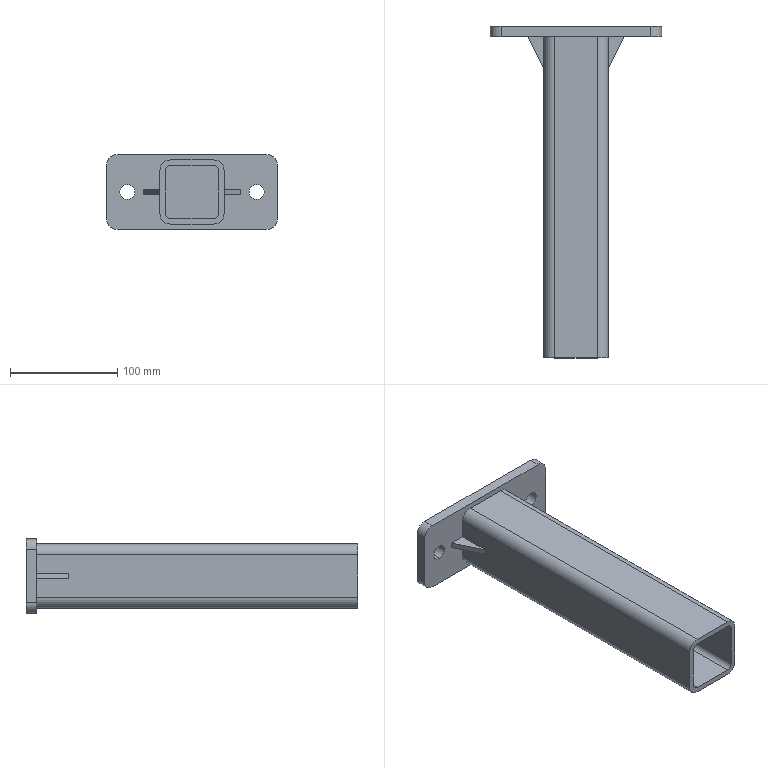Part | STEP file | MOUNTING_BOTTOM_PROFILEV11_Default<Machined> | 4 solids | 42 faces | box 160 x 310 x 70 mm | volume 420999 mm3 | plane 26 | cylinder 16 | commonest cylinder face diameters 20 x8 10 x4 14 x4